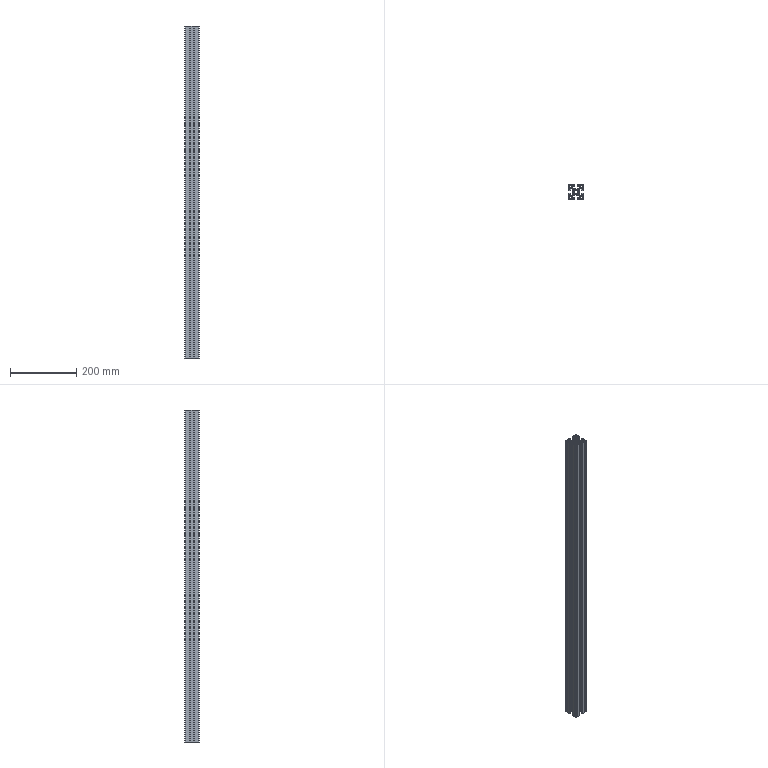Part | SolidWorks | features Extrusion 1 | 1 solid | 236 faces | box 45 x 45 x 1000 mm | volume 638120 mm3 | plane 178 | cylinder 58 | commonest cylinder face diameters 2 x36 3 x10 12 x8 4 x4